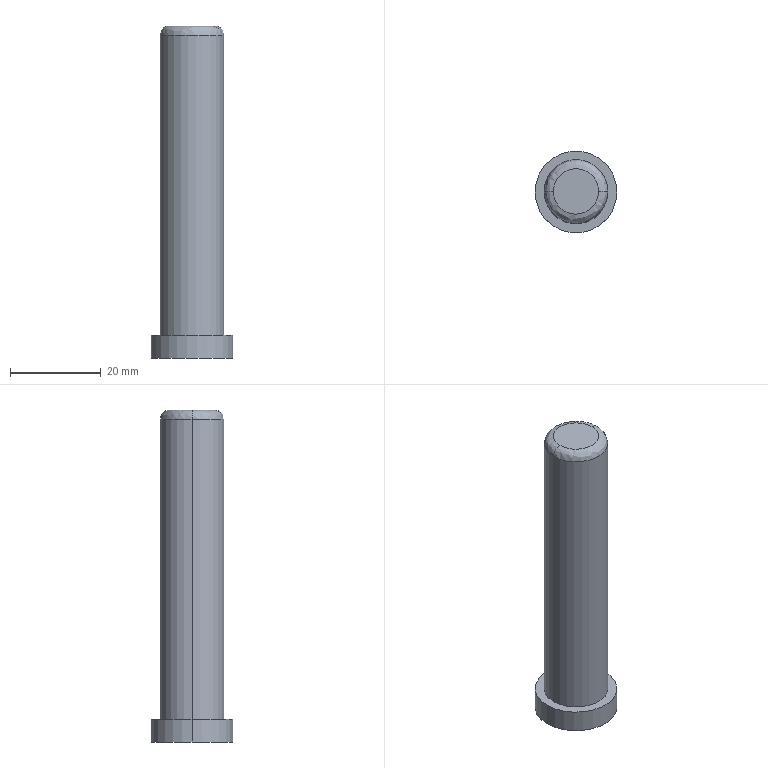Part | STEP file | COT DAN HUONG14X73 | 1 solid | 9 faces | box 18 x 18 x 73 mm | volume 11705 mm3 | cylinder 4 | plane 3 | spline 2 | commonest cylinder face diameters 14 x2 18 x2
STEP:
#1=CARTESIAN_POINT('',(0.,0.,0.));
#2=DIRECTION('',(0.,0.,1.));
#3=DIRECTION('',(1.,0.,0.));
#4=AXIS2_PLACEMENT_3D('',#1,#2,#3);
#5=CARTESIAN_POINT('',(7.,0.,71.));
#6=VERTEX_POINT('',#5);
#7=CARTESIAN_POINT('',(-7.,0.,71.));
#8=VERTEX_POINT('',#7);
#9=CARTESIAN_POINT('',(0.,0.,71.));
#10=DIRECTION('',(0.,0.,-1.));
#11=DIRECTION('',(1.,0.,0.));
#12=AXIS2_PLACEMENT_3D('',#9,#10,#11);
#13=CIRCLE('',#12,7.);
#14=CARTESIAN_POINT('',(7.,0.,71.));
#15=CARTESIAN_POINT('',(7.,-14.,71.));
#16=CARTESIAN_POINT('',(-7.,-14.,71.));
#17=CARTESIAN_POINT('',(-7.,0.,71.));
#18=CARTESIAN_POINT('',(7.,0.,72.172));
#19=CARTESIAN_POINT('',(7.,-14.,72.172));
#20=CARTESIAN_POINT('',(-7.,-14.,72.172));
#21=CARTESIAN_POINT('',(-7.,0.,72.172));
#22=CARTESIAN_POINT('',(6.172,0.,73.));
#23=CARTESIAN_POINT('',(6.172,-12.343,73.));
#24=CARTESIAN_POINT('',(-6.172,-12.343,73.));
#25=CARTESIAN_POINT('',(-6.172,0.,73.));
#26=CARTESIAN_POINT('',(5.,0.,73.));
#27=CARTESIAN_POINT('',(5.,-10.,73.));
#28=CARTESIAN_POINT('',(-5.,-10.,73.));
#29=CARTESIAN_POINT('',(-5.,0.,73.));
#30=(BOUNDED_SURFACE()B_SPLINE_SURFACE(3,3,((#14,#15,#16,#17),(#18,#19,#20,#21),(#22,#23,#24,#25),(#26,#27,#28,#29)),.UNSPECIFIED.,.F.,.F.,.F.)B_SPLINE_SURFACE_WITH_KNOTS((4,4),(4,4),(0.,1.),(0.,1.),.PIECEWISE_BEZIER_KNOTS.)GEOMETRIC_REPRESENTATION_ITEM()RATIONAL_B_SPLINE_SURFACE(((1.,0.3333,0.3333,1.),(0.8047,0.2682,0.2682,0.8047),(0.8047,0.2682,0.2682,0.8047),(1.,0.3333,0.3333,1.)))REPRESENTATION_ITEM('')SURFACE());
#31=CARTESIAN_POINT('',(0.,0.));
#32=CARTESIAN_POINT('',(0.,0.02375));
#33=CARTESIAN_POINT('',(0.,0.06805));
#34=CARTESIAN_POINT('',(0.,0.1267));
#35=CARTESIAN_POINT('',(0.,0.1794));
#36=CARTESIAN_POINT('',(0.,0.2276));
#37=CARTESIAN_POINT('',(0.,0.2721));
#38=CARTESIAN_POINT('',(0.,0.3139));
#39=CARTESIAN_POINT('',(0.,0.3535));
#40=CARTESIAN_POINT('',(0.,0.3914));
#41=CARTESIAN_POINT('',(0.,0.4282));
#42=CARTESIAN_POINT('',(0.,0.4643));
#43=CARTESIAN_POINT('',(0.,0.5));
#44=CARTESIAN_POINT('',(0.,0.5357));
#45=CARTESIAN_POINT('',(0.,0.5718));
#46=CARTESIAN_POINT('',(0.,0.6086));
#47=CARTESIAN_POINT('',(0.,0.6465));
#48=CARTESIAN_POINT('',(0.,0.6861));
#49=CARTESIAN_POINT('',(0.,0.7279));
#50=CARTESIAN_POINT('',(0.,0.7724));
#51=CARTESIAN_POINT('',(0.,0.8206));
#52=CARTESIAN_POINT('',(0.,0.8733));
#53=CARTESIAN_POINT('',(0.,0.9319));
#54=CARTESIAN_POINT('',(0.,0.9763));
#55=CARTESIAN_POINT('',(0.,1.));
#56=B_SPLINE_CURVE_WITH_KNOTS('',3,(#31,#32,#33,#34,#35,#36,#37,#38,#39,#40,#41,#42,#43,#44,#45,#46,#47,#48,#49,#50,#51,#52,#53,#54,#55),.UNSPECIFIED.,.F.,.F.,(4,1,1,1,1,1,1,1,1,1,1,1,1,1,1,1,1,1,1,1,1,1,4),(0.,0.1428,0.2856,0.4284,0.5712,0.714,0.8568,0.9996,1.142,1.285,1.428,1.571,1.714,1.856,1.999,2.142,2.285,2.428,2.57,2.713,2.856,2.999,3.142),.QUASI_UNIFORM_KNOTS.);
#57=(GEOMETRIC_REPRESENTATION_CONTEXT(2)PARAMETRIC_REPRESENTATION_CONTEXT()REPRESENTATION_CONTEXT('',''));
#58=DEFINITIONAL_REPRESENTATION('',(#56),#57);
#59=PCURVE('',#30,#58);
#60=CARTESIAN_POINT('',(0.,0.,5.));
#61=DIRECTION('',(0.,0.,1.));
#62=DIRECTION('',(1.,0.,0.));
#63=AXIS2_PLACEMENT_3D('',#60,#61,#62);
#64=CYLINDRICAL_SURFACE('',#63,7.);
#65=CARTESIAN_POINT('',(6.283,66.));
#66=DIRECTION('',(-1.,0.));
#67=VECTOR('',#66,1.);
#68=LINE('',#65,#67);
#69=(GEOMETRIC_REPRESENTATION_CONTEXT(2)PARAMETRIC_REPRESENTATION_CONTEXT()REPRESENTATION_CONTEXT('',''));
#70=DEFINITIONAL_REPRESENTATION('',(#68),#69);
#71=PCURVE('',#64,#70);
#72=SURFACE_CURVE('',#13,(#59,#71),.PCURVE_S1.);
#73=EDGE_CURVE('',#6,#8,#72,.T.);
#74=ORIENTED_EDGE('',*,*,#73,.F.);
#75=CARTESIAN_POINT('',(5.,0.,73.));
#76=VERTEX_POINT('',#75);
#77=CARTESIAN_POINT('',(5.,0.,71.));
#78=DIRECTION('',(0.,-1.,0.));
#79=DIRECTION('',(1.,0.,0.));
#80=AXIS2_PLACEMENT_3D('',#77,#78,#79);
#81=CIRCLE('',#80,2.);
#82=CARTESIAN_POINT('',(0.,0.));
#83=CARTESIAN_POINT('',(0.01683,0.));
#84=CARTESIAN_POINT('',(0.04999,0.));
#85=CARTESIAN_POINT('',(0.09843,0.));
#86=CARTESIAN_POINT('',(0.1457,0.));
#87=CARTESIAN_POINT('',(0.192,0.));
#88=CARTESIAN_POINT('',(0.2375,0.));
#89=CARTESIAN_POINT('',(0.2823,0.));
#90=CARTESIAN_POINT('',(0.3265,0.));
#91=CARTESIAN_POINT('',(0.3703,0.));
#92=CARTESIAN_POINT('',(0.4137,0.));
#93=CARTESIAN_POINT('',(0.4569,0.));
#94=CARTESIAN_POINT('',(0.5,0.));
#95=CARTESIAN_POINT('',(0.5431,0.));
#96=CARTESIAN_POINT('',(0.5863,0.));
#97=CARTESIAN_POINT('',(0.6297,0.));
#98=CARTESIAN_POINT('',(0.6735,0.));
#99=CARTESIAN_POINT('',(0.7177,0.));
#100=CARTESIAN_POINT('',(0.7625,0.));
#101=CARTESIAN_POINT('',(0.808,0.));
#102=CARTESIAN_POINT('',(0.8543,0.));
#103=CARTESIAN_POINT('',(0.9016,0.));
#104=CARTESIAN_POINT('',(0.95,0.));
#105=CARTESIAN_POINT('',(0.9832,0.));
#106=CARTESIAN_POINT('',(1.,0.));
#107=B_SPLINE_CURVE_WITH_KNOTS('',3,(#82,#83,#84,#85,#86,#87,#88,#89,#90,#91,#92,#93,#94,#95,#96,#97,#98,#99,#100,#101,#102,#103,#104,#105,#106),.UNSPECIFIED.,.F.,.F.,(4,1,1,1,1,1,1,1,1,1,1,1,1,1,1,1,1,1,1,1,1,1,4),(0.,0.0714,0.1428,0.2142,0.2856,0.357,0.4284,0.4998,0.5712,0.6426,0.714,0.7854,0.8568,0.9282,0.9996,1.071,1.142,1.214,1.285,1.357,1.428,1.499,1.571),.QUASI_UNIFORM_KNOTS.);
#108=(GEOMETRIC_REPRESENTATION_CONTEXT(2)PARAMETRIC_REPRESENTATION_CONTEXT()REPRESENTATION_CONTEXT('',''));
#109=DEFINITIONAL_REPRESENTATION('',(#107),#108);
#110=PCURVE('',#30,#109);
#111=CARTESIAN_POINT('',(-7.,0.,71.));
#112=CARTESIAN_POINT('',(-7.,14.,71.));
#113=CARTESIAN_POINT('',(7.,14.,71.));
#114=CARTESIAN_POINT('',(7.,0.,71.));
#115=CARTESIAN_POINT('',(-7.,0.,72.172));
#116=CARTESIAN_POINT('',(-7.,14.,72.172));
#117=CARTESIAN_POINT('',(7.,14.,72.172));
#118=CARTESIAN_POINT('',(7.,0.,72.172));
#119=CARTESIAN_POINT('',(-6.172,0.,73.));
#120=CARTESIAN_POINT('',(-6.172,12.343,73.));
#121=CARTESIAN_POINT('',(6.172,12.343,73.));
#122=CARTESIAN_POINT('',(6.172,0.,73.));
#123=CARTESIAN_POINT('',(-5.,0.,73.));
#124=CARTESIAN_POINT('',(-5.,10.,73.));
#125=CARTESIAN_POINT('',(5.,10.,73.));
#126=CARTESIAN_POINT('',(5.,0.,73.));
#127=(BOUNDED_SURFACE()B_SPLINE_SURFACE(3,3,((#111,#112,#113,#114),(#115,#116,#117,#118),(#119,#120,#121,#122),(#123,#124,#125,#126)),.UNSPECIFIED.,.F.,.F.,.F.)B_SPLINE_SURFACE_WITH_KNOTS((4,4),(4,4),(0.,1.),(0.,1.),.PIECEWISE_BEZIER_KNOTS.)GEOMETRIC_REPRESENTATION_ITEM()RATIONAL_B_SPLINE_SURFACE(((1.,0.3333,0.3333,1.),(0.8047,0.2682,0.2682,0.8047),(0.8047,0.2682,0.2682,0.8047),(1.,0.3333,0.3333,1.)))REPRESENTATION_ITEM('')SURFACE());
#128=CARTESIAN_POINT('',(0.,1.));
#129=CARTESIAN_POINT('',(0.01683,1.));
#130=CARTESIAN_POINT('',(0.04999,1.));
#131=CARTESIAN_POINT('',(0.09843,1.));
#132=CARTESIAN_POINT('',(0.1457,1.));
#133=CARTESIAN_POINT('',(0.192,1.));
#134=CARTESIAN_POINT('',(0.2375,1.));
#135=CARTESIAN_POINT('',(0.2823,1.));
#136=CARTESIAN_POINT('',(0.3265,1.));
#137=CARTESIAN_POINT('',(0.3703,1.));
#138=CARTESIAN_POINT('',(0.4137,1.));
#139=CARTESIAN_POINT('',(0.4569,1.));
#140=CARTESIAN_POINT('',(0.5,1.));
#141=CARTESIAN_POINT('',(0.5431,1.));
#142=CARTESIAN_POINT('',(0.5863,1.));
#143=CARTESIAN_POINT('',(0.6297,1.));
#144=CARTESIAN_POINT('',(0.6735,1.));
#145=CARTESIAN_POINT('',(0.7177,1.));
#146=CARTESIAN_POINT('',(0.7625,1.));
#147=CARTESIAN_POINT('',(0.808,1.));
#148=CARTESIAN_POINT('',(0.8543,1.));
#149=CARTESIAN_POINT('',(0.9016,1.));
#150=CARTESIAN_POINT('',(0.95,1.));
#151=CARTESIAN_POINT('',(0.9832,1.));
#152=CARTESIAN_POINT('',(1.,1.));
#153=B_SPLINE_CURVE_WITH_KNOTS('',3,(#128,#129,#130,#131,#132,#133,#134,#135,#136,#137,#138,#139,#140,#141,#142,#143,#144,#145,#146,#147,#148,#149,#150,#151,#152),.UNSPECIFIED.,.F.,.F.,(4,1,1,1,1,1,1,1,1,1,1,1,1,1,1,1,1,1,1,1,1,1,4),(0.,0.0714,0.1428,0.2142,0.2856,0.357,0.4284,0.4998,0.5712,0.6426,0.714,0.7854,0.8568,0.9282,0.9996,1.071,1.142,1.214,1.285,1.357,1.428,1.499,1.571),.QUASI_UNIFORM_KNOTS.);
#154=(GEOMETRIC_REPRESENTATION_CONTEXT(2)PARAMETRIC_REPRESENTATION_CONTEXT()REPRESENTATION_CONTEXT('',''));
#155=DEFINITIONAL_REPRESENTATION('',(#153),#154);
#156=PCURVE('',#127,#155);
#157=SURFACE_CURVE('',#81,(#110,#156),.PCURVE_S1.);
#158=EDGE_CURVE('',#6,#76,#157,.T.);
#159=ORIENTED_EDGE('',*,*,#158,.T.);
#160=CARTESIAN_POINT('',(-5.,0.,73.));
#161=VERTEX_POINT('',#160);
#162=CARTESIAN_POINT('',(5.,0.,73.));
#163=CARTESIAN_POINT('',(5.,-10.,73.));
#164=CARTESIAN_POINT('',(-5.,-10.,73.));
#165=CARTESIAN_POINT('',(-5.,0.,73.));
#166=(BOUNDED_CURVE()B_SPLINE_CURVE(3,(#162,#163,#164,#165),.UNSPECIFIED.,.F.,.F.)B_SPLINE_CURVE_WITH_KNOTS((4,4),(0.,0.5),.PIECEWISE_BEZIER_KNOTS.)CURVE()GEOMETRIC_REPRESENTATION_ITEM()RATIONAL_B_SPLINE_CURVE((1.,0.3333,0.3333,1.))REPRESENTATION_ITEM(''));
#167=CARTESIAN_POINT('',(1.,0.));
#168=CARTESIAN_POINT('',(1.,1.));
#169=B_SPLINE_CURVE_WITH_KNOTS('',1,(#167,#168),.UNSPECIFIED.,.F.,.F.,(2,2),(0.,0.5),.PIECEWISE_BEZIER_KNOTS.);
#170=(GEOMETRIC_REPRESENTATION_CONTEXT(2)PARAMETRIC_REPRESENTATION_CONTEXT()REPRESENTATION_CONTEXT('',''));
#171=DEFINITIONAL_REPRESENTATION('',(#169),#170);
#172=PCURVE('',#30,#171);
#173=CARTESIAN_POINT('',(0.,0.,73.));
#174=DIRECTION('',(0.,0.,-1.));
#175=DIRECTION('',(-1.,0.,0.));
#176=AXIS2_PLACEMENT_3D('',#173,#174,#175);
#177=PLANE('',#176);
#178=CARTESIAN_POINT('',(-5.,0.));
#179=CARTESIAN_POINT('',(-5.,-10.));
#180=CARTESIAN_POINT('',(5.,-10.));
#181=CARTESIAN_POINT('',(5.,0.));
#182=(BOUNDED_CURVE()B_SPLINE_CURVE(3,(#178,#179,#180,#181),.UNSPECIFIED.,.F.,.F.)B_SPLINE_CURVE_WITH_KNOTS((4,4),(0.,0.5),.PIECEWISE_BEZIER_KNOTS.)CURVE()GEOMETRIC_REPRESENTATION_ITEM()RATIONAL_B_SPLINE_CURVE((1.,0.3333,0.3333,1.))REPRESENTATION_ITEM(''));
#183=(GEOMETRIC_REPRESENTATION_CONTEXT(2)PARAMETRIC_REPRESENTATION_CONTEXT()REPRESENTATION_CONTEXT('',''));
#184=DEFINITIONAL_REPRESENTATION('',(#182),#183);
#185=PCURVE('',#177,#184);
#186=SURFACE_CURVE('',#166,(#172,#185),.PCURVE_S1.);
#187=EDGE_CURVE('',#76,#161,#186,.T.);
#188=ORIENTED_EDGE('',*,*,#187,.T.);
#189=CARTESIAN_POINT('',(-5.,0.,71.));
#190=DIRECTION('',(0.,1.,0.));
#191=DIRECTION('',(-1.,0.,0.));
#192=AXIS2_PLACEMENT_3D('',#189,#190,#191);
#193=CIRCLE('',#192,2.);
#194=CARTESIAN_POINT('',(0.,1.));
#195=CARTESIAN_POINT('',(0.01683,1.));
#196=CARTESIAN_POINT('',(0.04999,1.));
#197=CARTESIAN_POINT('',(0.09843,1.));
#198=CARTESIAN_POINT('',(0.1457,1.));
#199=CARTESIAN_POINT('',(0.192,1.));
#200=CARTESIAN_POINT('',(0.2375,1.));
#201=CARTESIAN_POINT('',(0.2823,1.));
#202=CARTESIAN_POINT('',(0.3265,1.));
#203=CARTESIAN_POINT('',(0.3703,1.));
#204=CARTESIAN_POINT('',(0.4137,1.));
#205=CARTESIAN_POINT('',(0.4569,1.));
#206=CARTESIAN_POINT('',(0.5,1.));
#207=CARTESIAN_POINT('',(0.5431,1.));
#208=CARTESIAN_POINT('',(0.5863,1.));
#209=CARTESIAN_POINT('',(0.6297,1.));
#210=CARTESIAN_POINT('',(0.6735,1.));
#211=CARTESIAN_POINT('',(0.7177,1.));
#212=CARTESIAN_POINT('',(0.7625,1.));
#213=CARTESIAN_POINT('',(0.808,1.));
#214=CARTESIAN_POINT('',(0.8543,1.));
#215=CARTESIAN_POINT('',(0.9016,1.));
#216=CARTESIAN_POINT('',(0.95,1.));
#217=CARTESIAN_POINT('',(0.9832,1.));
#218=CARTESIAN_POINT('',(1.,1.));
#219=B_SPLINE_CURVE_WITH_KNOTS('',3,(#194,#195,#196,#197,#198,#199,#200,#201,#202,#203,#204,#205,#206,#207,#208,#209,#210,#211,#212,#213,#214,#215,#216,#217,#218),.UNSPECIFIED.,.F.,.F.,(4,1,1,1,1,1,1,1,1,1,1,1,1,1,1,1,1,1,1,1,1,1,4),(0.,0.0714,0.1428,0.2142,0.2856,0.357,0.4284,0.4998,0.5712,0.6426,0.714,0.7854,0.8568,0.9282,0.9996,1.071,1.142,1.214,1.285,1.357,1.428,1.499,1.571),.QUASI_UNIFORM_KNOTS.);
#220=(GEOMETRIC_REPRESENTATION_CONTEXT(2)PARAMETRIC_REPRESENTATION_CONTEXT()REPRESENTATION_CONTEXT('',''));
#221=DEFINITIONAL_REPRESENTATION('',(#219),#220);
#222=PCURVE('',#30,#221);
#223=CARTESIAN_POINT('',(0.,0.));
#224=CARTESIAN_POINT('',(0.01683,0.));
#225=CARTESIAN_POINT('',(0.04999,0.));
#226=CARTESIAN_POINT('',(0.09843,0.));
#227=CARTESIAN_POINT('',(0.1457,0.));
#228=CARTESIAN_POINT('',(0.192,0.));
#229=CARTESIAN_POINT('',(0.2375,0.));
#230=CARTESIAN_POINT('',(0.2823,0.));
#231=CARTESIAN_POINT('',(0.3265,0.));
#232=CARTESIAN_POINT('',(0.3703,0.));
#233=CARTESIAN_POINT('',(0.4137,0.));
#234=CARTESIAN_POINT('',(0.4569,0.));
#235=CARTESIAN_POINT('',(0.5,0.));
#236=CARTESIAN_POINT('',(0.5431,0.));
#237=CARTESIAN_POINT('',(0.5863,0.));
#238=CARTESIAN_POINT('',(0.6297,0.));
#239=CARTESIAN_POINT('',(0.6735,0.));
#240=CARTESIAN_POINT('',(0.7177,0.));
#241=CARTESIAN_POINT('',(0.7625,0.));
#242=CARTESIAN_POINT('',(0.808,0.));
#243=CARTESIAN_POINT('',(0.8543,0.));
#244=CARTESIAN_POINT('',(0.9016,0.));
#245=CARTESIAN_POINT('',(0.95,0.));
#246=CARTESIAN_POINT('',(0.9832,0.));
#247=CARTESIAN_POINT('',(1.,0.));
#248=B_SPLINE_CURVE_WITH_KNOTS('',3,(#223,#224,#225,#226,#227,#228,#229,#230,#231,#232,#233,#234,#235,#236,#237,#238,#239,#240,#241,#242,#243,#244,#245,#246,#247),.UNSPECIFIED.,.F.,.F.,(4,1,1,1,1,1,1,1,1,1,1,1,1,1,1,1,1,1,1,1,1,1,4),(0.,0.0714,0.1428,0.2142,0.2856,0.357,0.4284,0.4998,0.5712,0.6426,0.714,0.7854,0.8568,0.9282,0.9996,1.071,1.142,1.214,1.285,1.357,1.428,1.499,1.571),.QUASI_UNIFORM_KNOTS.);
#249=(GEOMETRIC_REPRESENTATION_CONTEXT(2)PARAMETRIC_REPRESENTATION_CONTEXT()REPRESENTATION_CONTEXT('',''));
#250=DEFINITIONAL_REPRESENTATION('',(#248),#249);
#251=PCURVE('',#127,#250);
#252=SURFACE_CURVE('',#193,(#222,#251),.PCURVE_S1.);
#253=EDGE_CURVE('',#8,#161,#252,.T.);
#254=ORIENTED_EDGE('',*,*,#253,.F.);
#255=EDGE_LOOP('',(#74,#159,#188,#254));
#256=FACE_BOUND('',#255,.T.);
#257=ADVANCED_FACE('',(#256),#30,.T.);
#258=CARTESIAN_POINT('',(7.,0.,5.));
#259=VERTEX_POINT('',#258);
#260=CARTESIAN_POINT('',(-7.,0.,5.));
#261=VERTEX_POINT('',#260);
#262=CARTESIAN_POINT('',(0.,0.,5.));
#263=DIRECTION('',(0.,0.,1.));
#264=DIRECTION('',(1.,0.,0.));
#265=AXIS2_PLACEMENT_3D('',#262,#263,#264);
#266=CIRCLE('',#265,7.);
#267=CARTESIAN_POINT('',(0.,0.,5.));
#268=DIRECTION('',(0.,0.,1.));
#269=DIRECTION('',(1.,0.,0.));
#270=AXIS2_PLACEMENT_3D('',#267,#268,#269);
#271=CYLINDRICAL_SURFACE('',#270,7.);
#272=CARTESIAN_POINT('',(0.,0.));
#273=DIRECTION('',(1.,0.));
#274=VECTOR('',#273,1.);
#275=LINE('',#272,#274);
#276=(GEOMETRIC_REPRESENTATION_CONTEXT(2)PARAMETRIC_REPRESENTATION_CONTEXT()REPRESENTATION_CONTEXT('',''));
#277=DEFINITIONAL_REPRESENTATION('',(#275),#276);
#278=PCURVE('',#271,#277);
#279=CARTESIAN_POINT('',(0.,0.,5.));
#280=DIRECTION('',(0.,0.,-1.));
#281=DIRECTION('',(-1.,0.,0.));
#282=AXIS2_PLACEMENT_3D('',#279,#280,#281);
#283=PLANE('',#282);
#284=CARTESIAN_POINT('',(-7.,0.));
#285=CARTESIAN_POINT('',(-7.,12.124));
#286=CARTESIAN_POINT('',(3.5,6.062));
#287=CARTESIAN_POINT('',(14.,0.));
#288=CARTESIAN_POINT('',(3.5,-6.062));
#289=CARTESIAN_POINT('',(-7.,-12.124));
#290=CARTESIAN_POINT('',(-7.,0.));
#291=(BOUNDED_CURVE()B_SPLINE_CURVE(2,(#284,#285,#286,#287,#288,#289,#290),.UNSPECIFIED.,.T.,.F.)B_SPLINE_CURVE_WITH_KNOTS((1,2,2,2,2,1),(-2.094,0.,2.094,4.189,6.283,8.378),.UNSPECIFIED.)CURVE()GEOMETRIC_REPRESENTATION_ITEM()RATIONAL_B_SPLINE_CURVE((1.,0.5,1.,0.5,1.,0.5,1.))REPRESENTATION_ITEM(''));
#292=(GEOMETRIC_REPRESENTATION_CONTEXT(2)PARAMETRIC_REPRESENTATION_CONTEXT()REPRESENTATION_CONTEXT('',''));
#293=DEFINITIONAL_REPRESENTATION('',(#291),#292);
#294=PCURVE('',#283,#293);
#295=SURFACE_CURVE('',#266,(#278,#294),.PCURVE_S1.);
#296=EDGE_CURVE('',#259,#261,#295,.T.);
#297=ORIENTED_EDGE('',*,*,#296,.T.);
#298=CARTESIAN_POINT('',(-7.,0.,5.));
#299=DIRECTION('',(0.,0.,1.));
#300=VECTOR('',#299,1.);
#301=LINE('',#298,#300);
#302=CARTESIAN_POINT('',(3.142,0.));
#303=DIRECTION('',(0.,1.));
#304=VECTOR('',#303,1.);
#305=LINE('',#302,#304);
#306=(GEOMETRIC_REPRESENTATION_CONTEXT(2)PARAMETRIC_REPRESENTATION_CONTEXT()REPRESENTATION_CONTEXT('',''));
#307=DEFINITIONAL_REPRESENTATION('',(#305),#306);
#308=PCURVE('',#271,#307);
#309=CARTESIAN_POINT('',(3.142,0.));
#310=DIRECTION('',(0.,1.));
#311=VECTOR('',#310,1.);
#312=LINE('',#309,#311);
#313=(GEOMETRIC_REPRESENTATION_CONTEXT(2)PARAMETRIC_REPRESENTATION_CONTEXT()REPRESENTATION_CONTEXT('',''));
#314=DEFINITIONAL_REPRESENTATION('',(#312),#313);
#315=PCURVE('',#64,#314);
#316=SURFACE_CURVE('',#301,(#308,#315),.PCURVE_S1.);
#317=EDGE_CURVE('',#261,#8,#316,.T.);
#318=ORIENTED_EDGE('',*,*,#317,.T.);
#319=CARTESIAN_POINT('',(0.,0.,71.));
#320=DIRECTION('',(0.,0.,-1.));
#321=DIRECTION('',(1.,0.,0.));
#322=AXIS2_PLACEMENT_3D('',#319,#320,#321);
#323=CIRCLE('',#322,7.);
#324=CARTESIAN_POINT('',(6.283,66.));
#325=DIRECTION('',(-1.,0.));
#326=VECTOR('',#325,1.);
#327=LINE('',#324,#326);
#328=(GEOMETRIC_REPRESENTATION_CONTEXT(2)PARAMETRIC_REPRESENTATION_CONTEXT()REPRESENTATION_CONTEXT('',''));
#329=DEFINITIONAL_REPRESENTATION('',(#327),#328);
#330=PCURVE('',#271,#329);
#331=CARTESIAN_POINT('',(0.,0.));
#332=CARTESIAN_POINT('',(0.,0.02375));
#333=CARTESIAN_POINT('',(0.,0.06805));
#334=CARTESIAN_POINT('',(0.,0.1267));
#335=CARTESIAN_POINT('',(0.,0.1794));
#336=CARTESIAN_POINT('',(0.,0.2276));
#337=CARTESIAN_POINT('',(0.,0.2721));
#338=CARTESIAN_POINT('',(0.,0.3139));
#339=CARTESIAN_POINT('',(0.,0.3535));
#340=CARTESIAN_POINT('',(0.,0.3914));
#341=CARTESIAN_POINT('',(0.,0.4282));
#342=CARTESIAN_POINT('',(0.,0.4643));
#343=CARTESIAN_POINT('',(0.,0.5));
#344=CARTESIAN_POINT('',(0.,0.5357));
#345=CARTESIAN_POINT('',(0.,0.5718));
#346=CARTESIAN_POINT('',(0.,0.6086));
#347=CARTESIAN_POINT('',(0.,0.6465));
#348=CARTESIAN_POINT('',(0.,0.6861));
#349=CARTESIAN_POINT('',(0.,0.7279));
#350=CARTESIAN_POINT('',(0.,0.7724));
#351=CARTESIAN_POINT('',(0.,0.8206));
#352=CARTESIAN_POINT('',(0.,0.8733));
#353=CARTESIAN_POINT('',(0.,0.9319));
#354=CARTESIAN_POINT('',(0.,0.9763));
#355=CARTESIAN_POINT('',(0.,1.));
#356=B_SPLINE_CURVE_WITH_KNOTS('',3,(#331,#332,#333,#334,#335,#336,#337,#338,#339,#340,#341,#342,#343,#344,#345,#346,#347,#348,#349,#350,#351,#352,#353,#354,#355),.UNSPECIFIED.,.F.,.F.,(4,1,1,1,1,1,1,1,1,1,1,1,1,1,1,1,1,1,1,1,1,1,4),(3.142,3.284,3.427,3.57,3.713,3.856,3.998,4.141,4.284,4.427,4.57,4.712,4.855,4.998,5.141,5.284,5.426,5.569,5.712,5.855,5.998,6.14,6.283),.QUASI_UNIFORM_KNOTS.);
#357=(GEOMETRIC_REPRESENTATION_CONTEXT(2)PARAMETRIC_REPRESENTATION_CONTEXT()REPRESENTATION_CONTEXT('',''));
#358=DEFINITIONAL_REPRESENTATION('',(#356),#357);
#359=PCURVE('',#127,#358);
#360=SURFACE_CURVE('',#323,(#330,#359),.PCURVE_S1.);
#361=EDGE_CURVE('',#8,#6,#360,.T.);
#362=ORIENTED_EDGE('',*,*,#361,.T.);
#363=CARTESIAN_POINT('',(7.,0.,5.));
#364=DIRECTION('',(0.,0.,1.));
#365=VECTOR('',#364,1.);
#366=LINE('',#363,#365);
#367=CARTESIAN_POINT('',(0.,0.));
#368=DIRECTION('',(0.,1.));
#369=VECTOR('',#368,1.);
#370=LINE('',#367,#369);
#371=(GEOMETRIC_REPRESENTATION_CONTEXT(2)PARAMETRIC_REPRESENTATION_CONTEXT()REPRESENTATION_CONTEXT('',''));
#372=DEFINITIONAL_REPRESENTATION('',(#370),#371);
#373=PCURVE('',#271,#372);
#374=CARTESIAN_POINT('',(6.283,0.));
#375=DIRECTION('',(0.,1.));
#376=VECTOR('',#375,1.);
#377=LINE('',#374,#376);
#378=(GEOMETRIC_REPRESENTATION_CONTEXT(2)PARAMETRIC_REPRESENTATION_CONTEXT()REPRESENTATION_CONTEXT('',''));
#379=DEFINITIONAL_REPRESENTATION('',(#377),#378);
#380=PCURVE('',#64,#379);
#381=SURFACE_CURVE('',#366,(#373,#380),.PCURVE_S1.);
#382=EDGE_CURVE('',#259,#6,#381,.T.);
#383=ORIENTED_EDGE('',*,*,#382,.F.);
#384=EDGE_LOOP('',(#297,#318,#362,#383));
#385=FACE_BOUND('',#384,.T.);
#386=ADVANCED_FACE('',(#385),#271,.T.);
#387=CARTESIAN_POINT('',(9.,0.,0.));
#388=VERTEX_POINT('',#387);
#389=CARTESIAN_POINT('',(-9.,0.,0.));
#390=VERTEX_POINT('',#389);
#391=CARTESIAN_POINT('',(0.,0.,0.));
#392=DIRECTION('',(0.,0.,1.));
#393=DIRECTION('',(1.,0.,0.));
#394=AXIS2_PLACEMENT_3D('',#391,#392,#393);
#395=CIRCLE('',#394,9.);
#396=CARTESIAN_POINT('',(0.,0.,0.));
#397=DIRECTION('',(0.,0.,1.));
#398=DIRECTION('',(1.,0.,0.));
#399=AXIS2_PLACEMENT_3D('',#396,#397,#398);
#400=CYLINDRICAL_SURFACE('',#399,9.);
#401=CARTESIAN_POINT('',(0.,0.));
#402=DIRECTION('',(1.,0.));
#403=VECTOR('',#402,1.);
#404=LINE('',#401,#403);
#405=(GEOMETRIC_REPRESENTATION_CONTEXT(2)PARAMETRIC_REPRESENTATION_CONTEXT()REPRESENTATION_CONTEXT('',''));
#406=DEFINITIONAL_REPRESENTATION('',(#404),#405);
#407=PCURVE('',#400,#406);
#408=CARTESIAN_POINT('',(0.,0.,0.));
#409=DIRECTION('',(0.,0.,-1.));
#410=DIRECTION('',(-1.,0.,0.));
#411=AXIS2_PLACEMENT_3D('',#408,#409,#410);
#412=PLANE('',#411);
#413=CARTESIAN_POINT('',(-9.,0.));
#414=CARTESIAN_POINT('',(-9.,15.588));
#415=CARTESIAN_POINT('',(4.5,7.794));
#416=CARTESIAN_POINT('',(18.,0.));
#417=CARTESIAN_POINT('',(4.5,-7.794));
#418=CARTESIAN_POINT('',(-9.,-15.588));
#419=CARTESIAN_POINT('',(-9.,0.));
#420=(BOUNDED_CURVE()B_SPLINE_CURVE(2,(#413,#414,#415,#416,#417,#418,#419),.UNSPECIFIED.,.T.,.F.)B_SPLINE_CURVE_WITH_KNOTS((1,2,2,2,2,1),(-2.094,0.,2.094,4.189,6.283,8.378),.UNSPECIFIED.)CURVE()GEOMETRIC_REPRESENTATION_ITEM()RATIONAL_B_SPLINE_CURVE((1.,0.5,1.,0.5,1.,0.5,1.))REPRESENTATION_ITEM(''));
#421=(GEOMETRIC_REPRESENTATION_CONTEXT(2)PARAMETRIC_REPRESENTATION_CONTEXT()REPRESENTATION_CONTEXT('',''));
#422=DEFINITIONAL_REPRESENTATION('',(#420),#421);
#423=PCURVE('',#412,#422);
#424=SURFACE_CURVE('',#395,(#407,#423),.PCURVE_S1.);
#425=EDGE_CURVE('',#388,#390,#424,.T.);
#426=ORIENTED_EDGE('',*,*,#425,.T.);
#427=CARTESIAN_POINT('',(-9.,0.,5.));
#428=VERTEX_POINT('',#427);
#429=CARTESIAN_POINT('',(-9.,0.,0.));
#430=DIRECTION('',(0.,0.,1.));
#431=VECTOR('',#430,1.);
#432=LINE('',#429,#431);
#433=CARTESIAN_POINT('',(3.142,0.));
#434=DIRECTION('',(0.,1.));
#435=VECTOR('',#434,1.);
#436=LINE('',#433,#435);
#437=(GEOMETRIC_REPRESENTATION_CONTEXT(2)PARAMETRIC_REPRESENTATION_CONTEXT()REPRESENTATION_CONTEXT('',''));
#438=DEFINITIONAL_REPRESENTATION('',(#436),#437);
#439=PCURVE('',#400,#438);
#440=CARTESIAN_POINT('',(0.,0.,0.));
#441=DIRECTION('',(0.,0.,1.));
#442=DIRECTION('',(1.,0.,0.));
#443=AXIS2_PLACEMENT_3D('',#440,#441,#442);
#444=CYLINDRICAL_SURFACE('',#443,9.);
#445=CARTESIAN_POINT('',(3.142,0.));
#446=DIRECTION('',(0.,1.));
#447=VECTOR('',#446,1.);
#448=LINE('',#445,#447);
#449=(GEOMETRIC_REPRESENTATION_CONTEXT(2)PARAMETRIC_REPRESENTATION_CONTEXT()REPRESENTATION_CONTEXT('',''));
#450=DEFINITIONAL_REPRESENTATION('',(#448),#449);
#451=PCURVE('',#444,#450);
#452=SURFACE_CURVE('',#432,(#439,#451),.PCURVE_S1.);
#453=EDGE_CURVE('',#390,#428,#452,.T.);
#454=ORIENTED_EDGE('',*,*,#453,.T.);
#455=CARTESIAN_POINT('',(9.,0.,5.));
#456=VERTEX_POINT('',#455);
#457=CARTESIAN_POINT('',(0.,0.,5.));
#458=DIRECTION('',(0.,0.,-1.));
#459=DIRECTION('',(1.,0.,0.));
#460=AXIS2_PLACEMENT_3D('',#457,#458,#459);
#461=CIRCLE('',#460,9.);
#462=CARTESIAN_POINT('',(6.283,5.));
#463=DIRECTION('',(-1.,0.));
#464=VECTOR('',#463,1.);
#465=LINE('',#462,#464);
#466=(GEOMETRIC_REPRESENTATION_CONTEXT(2)PARAMETRIC_REPRESENTATION_CONTEXT()REPRESENTATION_CONTEXT('',''));
#467=DEFINITIONAL_REPRESENTATION('',(#465),#466);
#468=PCURVE('',#400,#467);
#469=CARTESIAN_POINT('',(0.,0.));
#470=DIRECTION('',(-1.,0.));
#471=AXIS2_PLACEMENT_2D('',#469,#470);
#472=CIRCLE('',#471,9.);
#473=(GEOMETRIC_REPRESENTATION_CONTEXT(2)PARAMETRIC_REPRESENTATION_CONTEXT()REPRESENTATION_CONTEXT('',''));
#474=DEFINITIONAL_REPRESENTATION('',(#472),#473);
#475=PCURVE('',#283,#474);
#476=SURFACE_CURVE('',#461,(#468,#475),.PCURVE_S1.);
#477=EDGE_CURVE('',#428,#456,#476,.T.);
#478=ORIENTED_EDGE('',*,*,#477,.T.);
#479=CARTESIAN_POINT('',(9.,0.,0.));
#480=DIRECTION('',(0.,0.,1.));
#481=VECTOR('',#480,1.);
#482=LINE('',#479,#481);
#483=CARTESIAN_POINT('',(0.,0.));
#484=DIRECTION('',(0.,1.));
#485=VECTOR('',#484,1.);
#486=LINE('',#483,#485);
#487=(GEOMETRIC_REPRESENTATION_CONTEXT(2)PARAMETRIC_REPRESENTATION_CONTEXT()REPRESENTATION_CONTEXT('',''));
#488=DEFINITIONAL_REPRESENTATION('',(#486),#487);
#489=PCURVE('',#400,#488);
#490=CARTESIAN_POINT('',(6.283,0.));
#491=DIRECTION('',(0.,1.));
#492=VECTOR('',#491,1.);
#493=LINE('',#490,#492);
#494=(GEOMETRIC_REPRESENTATION_CONTEXT(2)PARAMETRIC_REPRESENTATION_CONTEXT()REPRESENTATION_CONTEXT('',''));
#495=DEFINITIONAL_REPRESENTATION('',(#493),#494);
#496=PCURVE('',#444,#495);
#497=SURFACE_CURVE('',#482,(#489,#496),.PCURVE_S1.);
#498=EDGE_CURVE('',#388,#456,#497,.T.);
#499=ORIENTED_EDGE('',*,*,#498,.F.);
#500=EDGE_LOOP('',(#426,#454,#478,#499));
#501=FACE_BOUND('',#500,.T.);
#502=ADVANCED_FACE('',(#501),#400,.T.);
#503=ORIENTED_EDGE('',*,*,#317,.F.);
#504=CARTESIAN_POINT('',(0.,0.,5.));
#505=DIRECTION('',(0.,0.,1.));
#506=DIRECTION('',(1.,0.,0.));
#507=AXIS2_PLACEMENT_3D('',#504,#505,#506);
#508=CIRCLE('',#507,7.);
#509=CARTESIAN_POINT('',(0.,0.));
#510=DIRECTION('',(1.,0.));
#511=VECTOR('',#510,1.);
#512=LINE('',#509,#511);
#513=(GEOMETRIC_REPRESENTATION_CONTEXT(2)PARAMETRIC_REPRESENTATION_CONTEXT()REPRESENTATION_CONTEXT('',''));
#514=DEFINITIONAL_REPRESENTATION('',(#512),#513);
#515=PCURVE('',#64,#514);
#516=CARTESIAN_POINT('',(-7.,0.));
#517=CARTESIAN_POINT('',(-7.,12.124));
#518=CARTESIAN_POINT('',(3.5,6.062));
#519=CARTESIAN_POINT('',(14.,0.));
#520=CARTESIAN_POINT('',(3.5,-6.062));
#521=CARTESIAN_POINT('',(-7.,-12.124));
#522=CARTESIAN_POINT('',(-7.,0.));
#523=(BOUNDED_CURVE()B_SPLINE_CURVE(2,(#516,#517,#518,#519,#520,#521,#522),.UNSPECIFIED.,.T.,.F.)B_SPLINE_CURVE_WITH_KNOTS((1,2,2,2,2,1),(-2.094,0.,2.094,4.189,6.283,8.378),.UNSPECIFIED.)CURVE()GEOMETRIC_REPRESENTATION_ITEM()RATIONAL_B_SPLINE_CURVE((1.,0.5,1.,0.5,1.,0.5,1.))REPRESENTATION_ITEM(''));
#524=(GEOMETRIC_REPRESENTATION_CONTEXT(2)PARAMETRIC_REPRESENTATION_CONTEXT()REPRESENTATION_CONTEXT('',''));
#525=DEFINITIONAL_REPRESENTATION('',(#523),#524);
#526=PCURVE('',#283,#525);
#527=SURFACE_CURVE('',#508,(#515,#526),.PCURVE_S1.);
#528=EDGE_CURVE('',#261,#259,#527,.T.);
#529=ORIENTED_EDGE('',*,*,#528,.T.);
#530=ORIENTED_EDGE('',*,*,#382,.T.);
#531=ORIENTED_EDGE('',*,*,#73,.T.);
#532=EDGE_LOOP('',(#503,#529,#530,#531));
#533=FACE_BOUND('',#532,.T.);
#534=ADVANCED_FACE('',(#533),#64,.T.);
#535=ORIENTED_EDGE('',*,*,#158,.F.);
#536=ORIENTED_EDGE('',*,*,#361,.F.);
#537=ORIENTED_EDGE('',*,*,#253,.T.);
#538=CARTESIAN_POINT('',(-5.,0.,73.));
#539=CARTESIAN_POINT('',(-5.,10.,73.));
#540=CARTESIAN_POINT('',(5.,10.,73.));
#541=CARTESIAN_POINT('',(5.,0.,73.));
#542=(BOUNDED_CURVE()B_SPLINE_CURVE(3,(#538,#539,#540,#541),.UNSPECIFIED.,.F.,.F.)B_SPLINE_CURVE_WITH_KNOTS((4,4),(0.5,1.),.PIECEWISE_BEZIER_KNOTS.)CURVE()GEOMETRIC_REPRESENTATION_ITEM()RATIONAL_B_SPLINE_CURVE((1.,0.3333,0.3333,1.))REPRESENTATION_ITEM(''));
#543=CARTESIAN_POINT('',(1.,0.));
#544=CARTESIAN_POINT('',(1.,1.));
#545=B_SPLINE_CURVE_WITH_KNOTS('',1,(#543,#544),.UNSPECIFIED.,.F.,.F.,(2,2),(0.5,1.),.PIECEWISE_BEZIER_KNOTS.);
#546=(GEOMETRIC_REPRESENTATION_CONTEXT(2)PARAMETRIC_REPRESENTATION_CONTEXT()REPRESENTATION_CONTEXT('',''));
#547=DEFINITIONAL_REPRESENTATION('',(#545),#546);
#548=PCURVE('',#127,#547);
#549=CARTESIAN_POINT('',(5.,0.));
#550=CARTESIAN_POINT('',(5.,10.));
#551=CARTESIAN_POINT('',(-5.,10.));
#552=CARTESIAN_POINT('',(-5.,0.));
#553=(BOUNDED_CURVE()B_SPLINE_CURVE(3,(#549,#550,#551,#552),.UNSPECIFIED.,.F.,.F.)B_SPLINE_CURVE_WITH_KNOTS((4,4),(0.5,1.),.PIECEWISE_BEZIER_KNOTS.)CURVE()GEOMETRIC_REPRESENTATION_ITEM()RATIONAL_B_SPLINE_CURVE((1.,0.3333,0.3333,1.))REPRESENTATION_ITEM(''));
#554=(GEOMETRIC_REPRESENTATION_CONTEXT(2)PARAMETRIC_REPRESENTATION_CONTEXT()REPRESENTATION_CONTEXT('',''));
#555=DEFINITIONAL_REPRESENTATION('',(#553),#554);
#556=PCURVE('',#177,#555);
#557=SURFACE_CURVE('',#542,(#548,#556),.PCURVE_S1.);
#558=EDGE_CURVE('',#161,#76,#557,.T.);
#559=ORIENTED_EDGE('',*,*,#558,.T.);
#560=EDGE_LOOP('',(#535,#536,#537,#559));
#561=FACE_BOUND('',#560,.T.);
#562=ADVANCED_FACE('',(#561),#127,.T.);
#563=ORIENTED_EDGE('',*,*,#296,.F.);
#564=ORIENTED_EDGE('',*,*,#528,.F.);
#565=EDGE_LOOP('',(#563,#564));
#566=FACE_BOUND('',#565,.T.);
#567=CARTESIAN_POINT('',(0.,0.,5.));
#568=DIRECTION('',(0.,0.,-1.));
#569=DIRECTION('',(1.,0.,0.));
#570=AXIS2_PLACEMENT_3D('',#567,#568,#569);
#571=CIRCLE('',#570,9.);
#572=CARTESIAN_POINT('',(0.,0.));
#573=DIRECTION('',(-1.,0.));
#574=AXIS2_PLACEMENT_2D('',#572,#573);
#575=CIRCLE('',#574,9.);
#576=(GEOMETRIC_REPRESENTATION_CONTEXT(2)PARAMETRIC_REPRESENTATION_CONTEXT()REPRESENTATION_CONTEXT('',''));
#577=DEFINITIONAL_REPRESENTATION('',(#575),#576);
#578=PCURVE('',#283,#577);
#579=CARTESIAN_POINT('',(6.283,5.));
#580=DIRECTION('',(-1.,0.));
#581=VECTOR('',#580,1.);
#582=LINE('',#579,#581);
#583=(GEOMETRIC_REPRESENTATION_CONTEXT(2)PARAMETRIC_REPRESENTATION_CONTEXT()REPRESENTATION_CONTEXT('',''));
#584=DEFINITIONAL_REPRESENTATION('',(#582),#583);
#585=PCURVE('',#444,#584);
#586=SURFACE_CURVE('',#571,(#578,#585),.PCURVE_S1.);
#587=EDGE_CURVE('',#456,#428,#586,.T.);
#588=ORIENTED_EDGE('',*,*,#587,.F.);
#589=ORIENTED_EDGE('',*,*,#477,.F.);
#590=EDGE_LOOP('',(#588,#589));
#591=FACE_BOUND('',#590,.T.);
#592=ADVANCED_FACE('',(#566,#591),#283,.F.);
#593=ORIENTED_EDGE('',*,*,#558,.F.);
#594=ORIENTED_EDGE('',*,*,#187,.F.);
#595=EDGE_LOOP('',(#593,#594));
#596=FACE_BOUND('',#595,.T.);
#597=ADVANCED_FACE('',(#596),#177,.F.);
#598=ORIENTED_EDGE('',*,*,#453,.F.);
#599=CARTESIAN_POINT('',(0.,0.,0.));
#600=DIRECTION('',(0.,0.,1.));
#601=DIRECTION('',(1.,0.,0.));
#602=AXIS2_PLACEMENT_3D('',#599,#600,#601);
#603=CIRCLE('',#602,9.);
#604=CARTESIAN_POINT('',(0.,0.));
#605=DIRECTION('',(1.,0.));
#606=VECTOR('',#605,1.);
#607=LINE('',#604,#606);
#608=(GEOMETRIC_REPRESENTATION_CONTEXT(2)PARAMETRIC_REPRESENTATION_CONTEXT()REPRESENTATION_CONTEXT('',''));
#609=DEFINITIONAL_REPRESENTATION('',(#607),#608);
#610=PCURVE('',#444,#609);
#611=CARTESIAN_POINT('',(-9.,0.));
#612=CARTESIAN_POINT('',(-9.,15.588));
#613=CARTESIAN_POINT('',(4.5,7.794));
#614=CARTESIAN_POINT('',(18.,0.));
#615=CARTESIAN_POINT('',(4.5,-7.794));
#616=CARTESIAN_POINT('',(-9.,-15.588));
#617=CARTESIAN_POINT('',(-9.,0.));
#618=(BOUNDED_CURVE()B_SPLINE_CURVE(2,(#611,#612,#613,#614,#615,#616,#617),.UNSPECIFIED.,.T.,.F.)B_SPLINE_CURVE_WITH_KNOTS((1,2,2,2,2,1),(-2.094,0.,2.094,4.189,6.283,8.378),.UNSPECIFIED.)CURVE()GEOMETRIC_REPRESENTATION_ITEM()RATIONAL_B_SPLINE_CURVE((1.,0.5,1.,0.5,1.,0.5,1.))REPRESENTATION_ITEM(''));
#619=(GEOMETRIC_REPRESENTATION_CONTEXT(2)PARAMETRIC_REPRESENTATION_CONTEXT()REPRESENTATION_CONTEXT('',''));
#620=DEFINITIONAL_REPRESENTATION('',(#618),#619);
#621=PCURVE('',#412,#620);
#622=SURFACE_CURVE('',#603,(#610,#621),.PCURVE_S1.);
#623=EDGE_CURVE('',#390,#388,#622,.T.);
#624=ORIENTED_EDGE('',*,*,#623,.T.);
#625=ORIENTED_EDGE('',*,*,#498,.T.);
#626=ORIENTED_EDGE('',*,*,#587,.T.);
#627=EDGE_LOOP('',(#598,#624,#625,#626));
#628=FACE_BOUND('',#627,.T.);
#629=ADVANCED_FACE('',(#628),#444,.T.);
#630=ORIENTED_EDGE('',*,*,#425,.F.);
#631=ORIENTED_EDGE('',*,*,#623,.F.);
#632=EDGE_LOOP('',(#630,#631));
#633=FACE_BOUND('',#632,.T.);
#634=ADVANCED_FACE('',(#633),#412,.T.);
#635=CLOSED_SHELL('',(#257,#386,#502,#534,#562,#592,#597,#629,#634));
#636=MANIFOLD_SOLID_BREP('',#635);
#637=(LENGTH_UNIT()NAMED_UNIT(*)SI_UNIT(.MILLI.,.METRE.));
#638=UNCERTAINTY_MEASURE_WITH_UNIT(LENGTH_MEASURE(0.0000001),#637,'','');
#639=(NAMED_UNIT(*)PLANE_ANGLE_UNIT()SI_UNIT($,.RADIAN.));
#640=(NAMED_UNIT(*)SI_UNIT($,.STERADIAN.)SOLID_ANGLE_UNIT());
#641=(GEOMETRIC_REPRESENTATION_CONTEXT(3)GLOBAL_UNCERTAINTY_ASSIGNED_CONTEXT((#638))GLOBAL_UNIT_ASSIGNED_CONTEXT((#637,#639,#640))REPRESENTATION_CONTEXT('',''));
#642=ADVANCED_BREP_SHAPE_REPRESENTATION('',(#4,#636),#641);